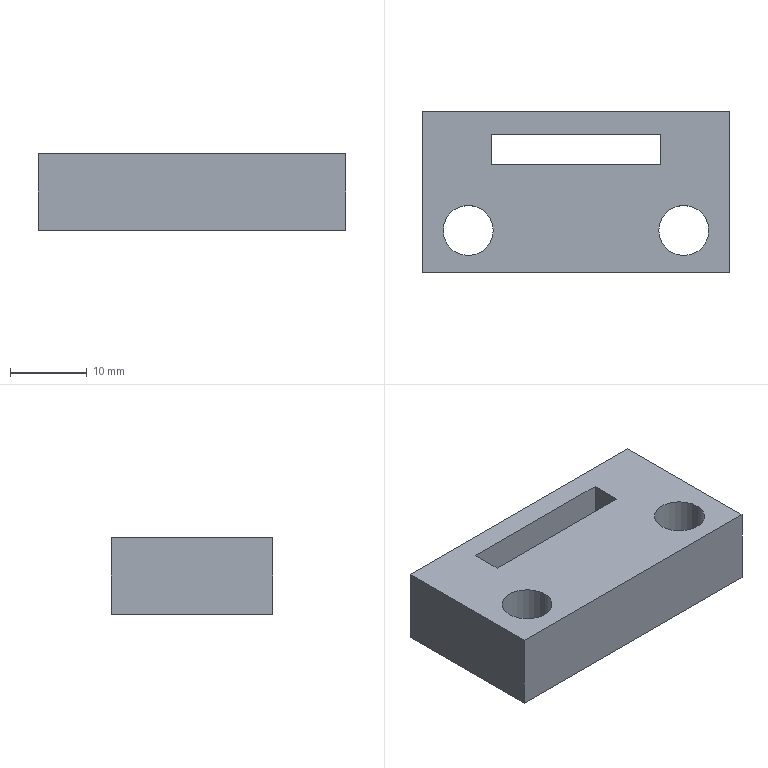Part | 1 solid | 15 faces | box 40 x 21 x 10 mm | volume 6698 mm3 | plane 11 | cylinder 4 | commonest cylinder face diameters 6.5 x4
STEP:
#1=CARTESIAN_POINT('',(10.75,0.,10.));
#2=VERTEX_POINT('',#1);
#3=CARTESIAN_POINT('',(17.25,0.,10.));
#4=VERTEX_POINT('',#3);
#5=CARTESIAN_POINT('',(14.,0.,10.));
#6=DIRECTION('',(0.,0.,1.));
#7=DIRECTION('',(1.,0.,0.));
#8=AXIS2_PLACEMENT_3D('',#5,#6,#7);
#9=CIRCLE('',#8,3.25);
#10=EDGE_CURVE('',#2,#4,#9,.T.);
#11=ORIENTED_EDGE('',*,*,#10,.T.);
#12=CARTESIAN_POINT('',(17.25,0.,0.));
#13=VERTEX_POINT('',#12);
#14=CARTESIAN_POINT('',(17.25,0.,10.));
#15=DIRECTION('',(0.,0.,-1.));
#16=VECTOR('',#15,1000.);
#17=LINE('',#14,#16);
#18=EDGE_CURVE('',#4,#13,#17,.T.);
#19=ORIENTED_EDGE('',*,*,#18,.T.);
#20=CARTESIAN_POINT('',(10.75,0.,0.));
#21=VERTEX_POINT('',#20);
#22=CARTESIAN_POINT('',(14.,0.,0.));
#23=DIRECTION('',(0.,0.,1.));
#24=DIRECTION('',(1.,0.,0.));
#25=AXIS2_PLACEMENT_3D('',#22,#23,#24);
#26=CIRCLE('',#25,3.25);
#27=EDGE_CURVE('',#21,#13,#26,.T.);
#28=ORIENTED_EDGE('',*,*,#27,.F.);
#29=CARTESIAN_POINT('',(10.75,0.,10.));
#30=DIRECTION('',(0.,0.,-1.));
#31=VECTOR('',#30,1000.);
#32=LINE('',#29,#31);
#33=EDGE_CURVE('',#2,#21,#32,.T.);
#34=ORIENTED_EDGE('',*,*,#33,.F.);
#35=EDGE_LOOP('',(#11,#19,#28,#34));
#36=FACE_OUTER_BOUND('',#35,.T.);
#37=CARTESIAN_POINT('',(14.,0.,10.));
#38=DIRECTION('',(0.,0.,-1.));
#39=DIRECTION('',(-1.,0.,0.));
#40=AXIS2_PLACEMENT_3D('',#37,#38,#39);
#41=CYLINDRICAL_SURFACE('',#40,3.25);
#42=ADVANCED_FACE('',(#36),#41,.F.);
#43=CARTESIAN_POINT('',(-17.25,0.,10.));
#44=VERTEX_POINT('',#43);
#45=CARTESIAN_POINT('',(-10.75,0.,10.));
#46=VERTEX_POINT('',#45);
#47=CARTESIAN_POINT('',(-14.,0.,10.));
#48=DIRECTION('',(0.,0.,1.));
#49=DIRECTION('',(1.,0.,0.));
#50=AXIS2_PLACEMENT_3D('',#47,#48,#49);
#51=CIRCLE('',#50,3.25);
#52=EDGE_CURVE('',#44,#46,#51,.T.);
#53=ORIENTED_EDGE('',*,*,#52,.T.);
#54=CARTESIAN_POINT('',(-10.75,0.,0.));
#55=VERTEX_POINT('',#54);
#56=CARTESIAN_POINT('',(-10.75,0.,10.));
#57=DIRECTION('',(0.,0.,-1.));
#58=VECTOR('',#57,1000.);
#59=LINE('',#56,#58);
#60=EDGE_CURVE('',#46,#55,#59,.T.);
#61=ORIENTED_EDGE('',*,*,#60,.T.);
#62=CARTESIAN_POINT('',(-17.25,0.,0.));
#63=VERTEX_POINT('',#62);
#64=CARTESIAN_POINT('',(-14.,0.,0.));
#65=DIRECTION('',(0.,0.,1.));
#66=DIRECTION('',(1.,0.,0.));
#67=AXIS2_PLACEMENT_3D('',#64,#65,#66);
#68=CIRCLE('',#67,3.25);
#69=EDGE_CURVE('',#63,#55,#68,.T.);
#70=ORIENTED_EDGE('',*,*,#69,.F.);
#71=CARTESIAN_POINT('',(-17.25,0.,10.));
#72=DIRECTION('',(0.,0.,-1.));
#73=VECTOR('',#72,1000.);
#74=LINE('',#71,#73);
#75=EDGE_CURVE('',#44,#63,#74,.T.);
#76=ORIENTED_EDGE('',*,*,#75,.F.);
#77=EDGE_LOOP('',(#53,#61,#70,#76));
#78=FACE_OUTER_BOUND('',#77,.T.);
#79=CARTESIAN_POINT('',(-14.,0.,10.));
#80=DIRECTION('',(0.,0.,-1.));
#81=DIRECTION('',(-1.,0.,0.));
#82=AXIS2_PLACEMENT_3D('',#79,#80,#81);
#83=CYLINDRICAL_SURFACE('',#82,3.25);
#84=ADVANCED_FACE('',(#78),#83,.F.);
#85=ORIENTED_EDGE('',*,*,#52,.F.);
#86=CARTESIAN_POINT('',(-14.,0.,10.));
#87=DIRECTION('',(0.,0.,1.));
#88=DIRECTION('',(1.,0.,0.));
#89=AXIS2_PLACEMENT_3D('',#86,#87,#88);
#90=CIRCLE('',#89,3.25);
#91=EDGE_CURVE('',#46,#44,#90,.T.);
#92=ORIENTED_EDGE('',*,*,#91,.F.);
#93=EDGE_LOOP('',(#85,#92));
#94=FACE_BOUND('',#93,.T.);
#95=CARTESIAN_POINT('',(20.,-5.5,10.));
#96=VERTEX_POINT('',#95);
#97=CARTESIAN_POINT('',(20.,15.5,10.));
#98=VERTEX_POINT('',#97);
#99=CARTESIAN_POINT('',(20.,-5.5,10.));
#100=DIRECTION('',(0.,1.,0.));
#101=VECTOR('',#100,1000.);
#102=LINE('',#99,#101);
#103=EDGE_CURVE('',#96,#98,#102,.T.);
#104=ORIENTED_EDGE('',*,*,#103,.T.);
#105=CARTESIAN_POINT('',(-20.,15.5,10.));
#106=VERTEX_POINT('',#105);
#107=CARTESIAN_POINT('',(-20.,15.5,10.));
#108=DIRECTION('',(-1.,0.,0.));
#109=VECTOR('',#108,1000.);
#110=LINE('',#107,#109);
#111=EDGE_CURVE('',#98,#106,#110,.T.);
#112=ORIENTED_EDGE('',*,*,#111,.T.);
#113=CARTESIAN_POINT('',(-20.,-5.5,10.));
#114=VERTEX_POINT('',#113);
#115=CARTESIAN_POINT('',(-20.,-5.5,10.));
#116=DIRECTION('',(0.,-1.,0.));
#117=VECTOR('',#116,1000.);
#118=LINE('',#115,#117);
#119=EDGE_CURVE('',#106,#114,#118,.T.);
#120=ORIENTED_EDGE('',*,*,#119,.T.);
#121=CARTESIAN_POINT('',(-20.,-5.5,10.));
#122=DIRECTION('',(1.,0.,0.));
#123=VECTOR('',#122,1000.);
#124=LINE('',#121,#123);
#125=EDGE_CURVE('',#114,#96,#124,.T.);
#126=ORIENTED_EDGE('',*,*,#125,.T.);
#127=EDGE_LOOP('',(#104,#112,#120,#126));
#128=FACE_OUTER_BOUND('',#127,.T.);
#129=ORIENTED_EDGE('',*,*,#10,.F.);
#130=CARTESIAN_POINT('',(14.,0.,10.));
#131=DIRECTION('',(0.,0.,1.));
#132=DIRECTION('',(1.,0.,0.));
#133=AXIS2_PLACEMENT_3D('',#130,#131,#132);
#134=CIRCLE('',#133,3.25);
#135=EDGE_CURVE('',#4,#2,#134,.T.);
#136=ORIENTED_EDGE('',*,*,#135,.F.);
#137=EDGE_LOOP('',(#129,#136));
#138=FACE_BOUND('',#137,.T.);
#139=CARTESIAN_POINT('',(-11.,8.5,10.));
#140=VERTEX_POINT('',#139);
#141=CARTESIAN_POINT('',(11.,8.5,10.));
#142=VERTEX_POINT('',#141);
#143=CARTESIAN_POINT('',(-11.,8.5,10.));
#144=DIRECTION('',(1.,0.,0.));
#145=VECTOR('',#144,1000.);
#146=LINE('',#143,#145);
#147=EDGE_CURVE('',#140,#142,#146,.T.);
#148=ORIENTED_EDGE('',*,*,#147,.F.);
#149=CARTESIAN_POINT('',(-11.,12.5,10.));
#150=VERTEX_POINT('',#149);
#151=CARTESIAN_POINT('',(-11.,12.5,10.));
#152=DIRECTION('',(0.,-1.,0.));
#153=VECTOR('',#152,1000.);
#154=LINE('',#151,#153);
#155=EDGE_CURVE('',#150,#140,#154,.T.);
#156=ORIENTED_EDGE('',*,*,#155,.F.);
#157=CARTESIAN_POINT('',(11.,12.5,10.));
#158=VERTEX_POINT('',#157);
#159=CARTESIAN_POINT('',(-11.,12.5,10.));
#160=DIRECTION('',(-1.,0.,0.));
#161=VECTOR('',#160,1000.);
#162=LINE('',#159,#161);
#163=EDGE_CURVE('',#158,#150,#162,.T.);
#164=ORIENTED_EDGE('',*,*,#163,.F.);
#165=CARTESIAN_POINT('',(11.,12.5,10.));
#166=DIRECTION('',(0.,1.,0.));
#167=VECTOR('',#166,1000.);
#168=LINE('',#165,#167);
#169=EDGE_CURVE('',#142,#158,#168,.T.);
#170=ORIENTED_EDGE('',*,*,#169,.F.);
#171=EDGE_LOOP('',(#148,#156,#164,#170));
#172=FACE_BOUND('',#171,.T.);
#173=CARTESIAN_POINT('',(0.,0.,10.));
#174=DIRECTION('',(0.,0.,-1.));
#175=DIRECTION('',(-1.,0.,0.));
#176=AXIS2_PLACEMENT_3D('',#173,#174,#175);
#177=PLANE('',#176);
#178=ADVANCED_FACE('',(#94,#128,#138,#172),#177,.F.);
#179=ORIENTED_EDGE('',*,*,#69,.T.);
#180=CARTESIAN_POINT('',(-14.,0.,0.));
#181=DIRECTION('',(0.,0.,1.));
#182=DIRECTION('',(1.,0.,0.));
#183=AXIS2_PLACEMENT_3D('',#180,#181,#182);
#184=CIRCLE('',#183,3.25);
#185=EDGE_CURVE('',#55,#63,#184,.T.);
#186=ORIENTED_EDGE('',*,*,#185,.T.);
#187=EDGE_LOOP('',(#179,#186));
#188=FACE_BOUND('',#187,.T.);
#189=CARTESIAN_POINT('',(20.,-5.5,0.));
#190=VERTEX_POINT('',#189);
#191=CARTESIAN_POINT('',(20.,15.5,0.));
#192=VERTEX_POINT('',#191);
#193=CARTESIAN_POINT('',(20.,-5.5,0.));
#194=DIRECTION('',(0.,1.,0.));
#195=VECTOR('',#194,1000.);
#196=LINE('',#193,#195);
#197=EDGE_CURVE('',#190,#192,#196,.T.);
#198=ORIENTED_EDGE('',*,*,#197,.F.);
#199=CARTESIAN_POINT('',(-20.,-5.5,0.));
#200=VERTEX_POINT('',#199);
#201=CARTESIAN_POINT('',(-20.,-5.5,0.));
#202=DIRECTION('',(1.,0.,0.));
#203=VECTOR('',#202,1000.);
#204=LINE('',#201,#203);
#205=EDGE_CURVE('',#200,#190,#204,.T.);
#206=ORIENTED_EDGE('',*,*,#205,.F.);
#207=CARTESIAN_POINT('',(-20.,15.5,0.));
#208=VERTEX_POINT('',#207);
#209=CARTESIAN_POINT('',(-20.,-5.5,0.));
#210=DIRECTION('',(0.,-1.,0.));
#211=VECTOR('',#210,1000.);
#212=LINE('',#209,#211);
#213=EDGE_CURVE('',#208,#200,#212,.T.);
#214=ORIENTED_EDGE('',*,*,#213,.F.);
#215=CARTESIAN_POINT('',(-20.,15.5,0.));
#216=DIRECTION('',(-1.,0.,0.));
#217=VECTOR('',#216,1000.);
#218=LINE('',#215,#217);
#219=EDGE_CURVE('',#192,#208,#218,.T.);
#220=ORIENTED_EDGE('',*,*,#219,.F.);
#221=EDGE_LOOP('',(#198,#206,#214,#220));
#222=FACE_OUTER_BOUND('',#221,.T.);
#223=ORIENTED_EDGE('',*,*,#27,.T.);
#224=CARTESIAN_POINT('',(14.,0.,0.));
#225=DIRECTION('',(0.,0.,1.));
#226=DIRECTION('',(1.,0.,0.));
#227=AXIS2_PLACEMENT_3D('',#224,#225,#226);
#228=CIRCLE('',#227,3.25);
#229=EDGE_CURVE('',#13,#21,#228,.T.);
#230=ORIENTED_EDGE('',*,*,#229,.T.);
#231=EDGE_LOOP('',(#223,#230));
#232=FACE_BOUND('',#231,.T.);
#233=CARTESIAN_POINT('',(-11.,5.613,0.));
#234=VERTEX_POINT('',#233);
#235=CARTESIAN_POINT('',(11.,5.613,0.));
#236=VERTEX_POINT('',#235);
#237=CARTESIAN_POINT('',(11.,5.613,0.));
#238=DIRECTION('',(1.,0.,0.));
#239=VECTOR('',#238,1000.);
#240=LINE('',#237,#239);
#241=EDGE_CURVE('',#234,#236,#240,.T.);
#242=ORIENTED_EDGE('',*,*,#241,.T.);
#243=CARTESIAN_POINT('',(11.,12.5,0.));
#244=VERTEX_POINT('',#243);
#245=CARTESIAN_POINT('',(11.,12.5,0.));
#246=DIRECTION('',(0.,1.,0.));
#247=VECTOR('',#246,1000.);
#248=LINE('',#245,#247);
#249=EDGE_CURVE('',#236,#244,#248,.T.);
#250=ORIENTED_EDGE('',*,*,#249,.T.);
#251=CARTESIAN_POINT('',(-11.,12.5,0.));
#252=VERTEX_POINT('',#251);
#253=CARTESIAN_POINT('',(-11.,12.5,0.));
#254=DIRECTION('',(-1.,0.,0.));
#255=VECTOR('',#254,1000.);
#256=LINE('',#253,#255);
#257=EDGE_CURVE('',#244,#252,#256,.T.);
#258=ORIENTED_EDGE('',*,*,#257,.T.);
#259=CARTESIAN_POINT('',(-11.,12.5,0.));
#260=DIRECTION('',(0.,-1.,0.));
#261=VECTOR('',#260,1000.);
#262=LINE('',#259,#261);
#263=EDGE_CURVE('',#252,#234,#262,.T.);
#264=ORIENTED_EDGE('',*,*,#263,.T.);
#265=EDGE_LOOP('',(#242,#250,#258,#264));
#266=FACE_BOUND('',#265,.T.);
#267=CARTESIAN_POINT('',(0.,0.,0.));
#268=DIRECTION('',(0.,0.,-1.));
#269=DIRECTION('',(-1.,0.,0.));
#270=AXIS2_PLACEMENT_3D('',#267,#268,#269);
#271=PLANE('',#270);
#272=ADVANCED_FACE('',(#188,#222,#232,#266),#271,.T.);
#273=ORIENTED_EDGE('',*,*,#197,.T.);
#274=CARTESIAN_POINT('',(20.,15.5,-41.231));
#275=DIRECTION('',(0.,0.,1.));
#276=VECTOR('',#275,1000.);
#277=LINE('',#274,#276);
#278=EDGE_CURVE('',#192,#98,#277,.T.);
#279=ORIENTED_EDGE('',*,*,#278,.T.);
#280=ORIENTED_EDGE('',*,*,#103,.F.);
#281=CARTESIAN_POINT('',(20.,-5.5,10.));
#282=DIRECTION('',(0.,0.,-1.));
#283=VECTOR('',#282,1000.);
#284=LINE('',#281,#283);
#285=EDGE_CURVE('',#96,#190,#284,.T.);
#286=ORIENTED_EDGE('',*,*,#285,.T.);
#287=EDGE_LOOP('',(#273,#279,#280,#286));
#288=FACE_OUTER_BOUND('',#287,.T.);
#289=CARTESIAN_POINT('',(20.,-5.5,10.));
#290=DIRECTION('',(-1.,0.,0.));
#291=DIRECTION('',(0.,0.,1.));
#292=AXIS2_PLACEMENT_3D('',#289,#290,#291);
#293=PLANE('',#292);
#294=ADVANCED_FACE('',(#288),#293,.F.);
#295=ORIENTED_EDGE('',*,*,#213,.T.);
#296=CARTESIAN_POINT('',(-20.,-5.5,10.));
#297=DIRECTION('',(0.,0.,-1.));
#298=VECTOR('',#297,1000.);
#299=LINE('',#296,#298);
#300=EDGE_CURVE('',#114,#200,#299,.T.);
#301=ORIENTED_EDGE('',*,*,#300,.F.);
#302=ORIENTED_EDGE('',*,*,#119,.F.);
#303=CARTESIAN_POINT('',(-20.,15.5,-41.231));
#304=DIRECTION('',(0.,0.,1.));
#305=VECTOR('',#304,1000.);
#306=LINE('',#303,#305);
#307=EDGE_CURVE('',#208,#106,#306,.T.);
#308=ORIENTED_EDGE('',*,*,#307,.F.);
#309=EDGE_LOOP('',(#295,#301,#302,#308));
#310=FACE_OUTER_BOUND('',#309,.T.);
#311=CARTESIAN_POINT('',(-20.,-5.5,10.));
#312=DIRECTION('',(1.,0.,0.));
#313=DIRECTION('',(0.,0.,-1.));
#314=AXIS2_PLACEMENT_3D('',#311,#312,#313);
#315=PLANE('',#314);
#316=ADVANCED_FACE('',(#310),#315,.F.);
#317=ORIENTED_EDGE('',*,*,#205,.T.);
#318=ORIENTED_EDGE('',*,*,#285,.F.);
#319=ORIENTED_EDGE('',*,*,#125,.F.);
#320=ORIENTED_EDGE('',*,*,#300,.T.);
#321=EDGE_LOOP('',(#317,#318,#319,#320));
#322=FACE_OUTER_BOUND('',#321,.T.);
#323=CARTESIAN_POINT('',(-20.,-5.5,10.));
#324=DIRECTION('',(0.,1.,0.));
#325=DIRECTION('',(0.,0.,1.));
#326=AXIS2_PLACEMENT_3D('',#323,#324,#325);
#327=PLANE('',#326);
#328=ADVANCED_FACE('',(#322),#327,.F.);
#329=ORIENTED_EDGE('',*,*,#60,.F.);
#330=ORIENTED_EDGE('',*,*,#91,.T.);
#331=ORIENTED_EDGE('',*,*,#75,.T.);
#332=ORIENTED_EDGE('',*,*,#185,.F.);
#333=EDGE_LOOP('',(#329,#330,#331,#332));
#334=FACE_OUTER_BOUND('',#333,.T.);
#335=CARTESIAN_POINT('',(-14.,0.,10.));
#336=DIRECTION('',(0.,0.,-1.));
#337=DIRECTION('',(-1.,0.,0.));
#338=AXIS2_PLACEMENT_3D('',#335,#336,#337);
#339=CYLINDRICAL_SURFACE('',#338,3.25);
#340=ADVANCED_FACE('',(#334),#339,.F.);
#341=ORIENTED_EDGE('',*,*,#18,.F.);
#342=ORIENTED_EDGE('',*,*,#135,.T.);
#343=ORIENTED_EDGE('',*,*,#33,.T.);
#344=ORIENTED_EDGE('',*,*,#229,.F.);
#345=EDGE_LOOP('',(#341,#342,#343,#344));
#346=FACE_OUTER_BOUND('',#345,.T.);
#347=CARTESIAN_POINT('',(14.,0.,10.));
#348=DIRECTION('',(0.,0.,-1.));
#349=DIRECTION('',(-1.,0.,0.));
#350=AXIS2_PLACEMENT_3D('',#347,#348,#349);
#351=CYLINDRICAL_SURFACE('',#350,3.25);
#352=ADVANCED_FACE('',(#346),#351,.F.);
#353=ORIENTED_EDGE('',*,*,#278,.F.);
#354=ORIENTED_EDGE('',*,*,#219,.T.);
#355=ORIENTED_EDGE('',*,*,#307,.T.);
#356=ORIENTED_EDGE('',*,*,#111,.F.);
#357=EDGE_LOOP('',(#353,#354,#355,#356));
#358=FACE_OUTER_BOUND('',#357,.T.);
#359=CARTESIAN_POINT('',(-20.,15.5,-41.231));
#360=DIRECTION('',(0.,1.,0.));
#361=DIRECTION('',(0.,0.,1.));
#362=AXIS2_PLACEMENT_3D('',#359,#360,#361);
#363=PLANE('',#362);
#364=ADVANCED_FACE('',(#358),#363,.T.);
#365=ORIENTED_EDGE('',*,*,#263,.F.);
#366=CARTESIAN_POINT('',(-11.,12.5,-41.231));
#367=DIRECTION('',(0.,0.,1.));
#368=VECTOR('',#367,1000.);
#369=LINE('',#366,#368);
#370=EDGE_CURVE('',#252,#150,#369,.T.);
#371=ORIENTED_EDGE('',*,*,#370,.T.);
#372=ORIENTED_EDGE('',*,*,#155,.T.);
#373=CARTESIAN_POINT('',(-11.,8.5,5.));
#374=VERTEX_POINT('',#373);
#375=CARTESIAN_POINT('',(-11.,8.5,-41.231));
#376=DIRECTION('',(0.,0.,1.));
#377=VECTOR('',#376,1000.);
#378=LINE('',#375,#377);
#379=EDGE_CURVE('',#374,#140,#378,.T.);
#380=ORIENTED_EDGE('',*,*,#379,.F.);
#381=CARTESIAN_POINT('',(-11.,-10.519,-27.941));
#382=DIRECTION('',(0.,-0.5,-0.866));
#383=VECTOR('',#382,1000.);
#384=LINE('',#381,#383);
#385=EDGE_CURVE('',#374,#234,#384,.T.);
#386=ORIENTED_EDGE('',*,*,#385,.T.);
#387=EDGE_LOOP('',(#365,#371,#372,#380,#386));
#388=FACE_OUTER_BOUND('',#387,.T.);
#389=CARTESIAN_POINT('',(-11.,12.5,-41.231));
#390=DIRECTION('',(-1.,0.,0.));
#391=DIRECTION('',(0.,-1.,0.));
#392=AXIS2_PLACEMENT_3D('',#389,#390,#391);
#393=PLANE('',#392);
#394=ADVANCED_FACE('',(#388),#393,.F.);
#395=ORIENTED_EDGE('',*,*,#257,.F.);
#396=CARTESIAN_POINT('',(11.,12.5,-41.231));
#397=DIRECTION('',(0.,0.,1.));
#398=VECTOR('',#397,1000.);
#399=LINE('',#396,#398);
#400=EDGE_CURVE('',#244,#158,#399,.T.);
#401=ORIENTED_EDGE('',*,*,#400,.T.);
#402=ORIENTED_EDGE('',*,*,#163,.T.);
#403=ORIENTED_EDGE('',*,*,#370,.F.);
#404=EDGE_LOOP('',(#395,#401,#402,#403));
#405=FACE_OUTER_BOUND('',#404,.T.);
#406=CARTESIAN_POINT('',(-11.,12.5,-41.231));
#407=DIRECTION('',(0.,1.,0.));
#408=DIRECTION('',(-1.,0.,0.));
#409=AXIS2_PLACEMENT_3D('',#406,#407,#408);
#410=PLANE('',#409);
#411=ADVANCED_FACE('',(#405),#410,.F.);
#412=ORIENTED_EDGE('',*,*,#249,.F.);
#413=CARTESIAN_POINT('',(11.,8.5,5.));
#414=VERTEX_POINT('',#413);
#415=CARTESIAN_POINT('',(11.,-10.519,-27.941));
#416=DIRECTION('',(0.,0.5,0.866));
#417=VECTOR('',#416,1000.);
#418=LINE('',#415,#417);
#419=EDGE_CURVE('',#236,#414,#418,.T.);
#420=ORIENTED_EDGE('',*,*,#419,.T.);
#421=CARTESIAN_POINT('',(11.,8.5,-41.231));
#422=DIRECTION('',(0.,0.,1.));
#423=VECTOR('',#422,1000.);
#424=LINE('',#421,#423);
#425=EDGE_CURVE('',#414,#142,#424,.T.);
#426=ORIENTED_EDGE('',*,*,#425,.T.);
#427=ORIENTED_EDGE('',*,*,#169,.T.);
#428=ORIENTED_EDGE('',*,*,#400,.F.);
#429=EDGE_LOOP('',(#412,#420,#426,#427,#428));
#430=FACE_OUTER_BOUND('',#429,.T.);
#431=CARTESIAN_POINT('',(11.,12.5,-41.231));
#432=DIRECTION('',(1.,0.,0.));
#433=DIRECTION('',(0.,1.,0.));
#434=AXIS2_PLACEMENT_3D('',#431,#432,#433);
#435=PLANE('',#434);
#436=ADVANCED_FACE('',(#430),#435,.F.);
#437=ORIENTED_EDGE('',*,*,#425,.F.);
#438=CARTESIAN_POINT('',(-11.,8.5,5.));
#439=DIRECTION('',(-1.,0.,0.));
#440=VECTOR('',#439,1000.);
#441=LINE('',#438,#440);
#442=EDGE_CURVE('',#414,#374,#441,.T.);
#443=ORIENTED_EDGE('',*,*,#442,.T.);
#444=ORIENTED_EDGE('',*,*,#379,.T.);
#445=ORIENTED_EDGE('',*,*,#147,.T.);
#446=EDGE_LOOP('',(#437,#443,#444,#445));
#447=FACE_OUTER_BOUND('',#446,.T.);
#448=CARTESIAN_POINT('',(-11.,8.5,-41.231));
#449=DIRECTION('',(0.,-1.,0.));
#450=DIRECTION('',(1.,0.,0.));
#451=AXIS2_PLACEMENT_3D('',#448,#449,#450);
#452=PLANE('',#451);
#453=ADVANCED_FACE('',(#447),#452,.F.);
#454=ORIENTED_EDGE('',*,*,#385,.F.);
#455=ORIENTED_EDGE('',*,*,#442,.F.);
#456=ORIENTED_EDGE('',*,*,#419,.F.);
#457=ORIENTED_EDGE('',*,*,#241,.F.);
#458=EDGE_LOOP('',(#454,#455,#456,#457));
#459=FACE_OUTER_BOUND('',#458,.T.);
#460=CARTESIAN_POINT('',(0.,5.613,0.));
#461=DIRECTION('',(0.,0.866,-0.5));
#462=DIRECTION('',(-1.,0.,0.));
#463=AXIS2_PLACEMENT_3D('',#460,#461,#462);
#464=PLANE('',#463);
#465=ADVANCED_FACE('',(#459),#464,.T.);
#466=CLOSED_SHELL('',(#42,#84,#178,#272,#294,#316,#328,#340,#352,#364,#394,#411,#436,#453,#465));
#467=MANIFOLD_SOLID_BREP('',#466);
#468=CARTESIAN_POINT('',(0.,0.,0.));
#469=DIRECTION('',(0.,0.,1.));
#470=DIRECTION('',(1.,0.,0.));
#471=AXIS2_PLACEMENT_3D('',#468,#469,#470);
#472=(LENGTH_UNIT()NAMED_UNIT(*)SI_UNIT(.MILLI.,.METRE.));
#473=UNCERTAINTY_MEASURE_WITH_UNIT(LENGTH_MEASURE(0.00001),#472,'','');
#474=(NAMED_UNIT(*)PLANE_ANGLE_UNIT()SI_UNIT($,.RADIAN.));
#475=(NAMED_UNIT(*)SI_UNIT($,.STERADIAN.)SOLID_ANGLE_UNIT());
#476=(GEOMETRIC_REPRESENTATION_CONTEXT(3)GLOBAL_UNCERTAINTY_ASSIGNED_CONTEXT((#473))GLOBAL_UNIT_ASSIGNED_CONTEXT((#472,#474,#475))REPRESENTATION_CONTEXT('',''));
#477=ADVANCED_BREP_SHAPE_REPRESENTATION('',(#467,#471),#476);